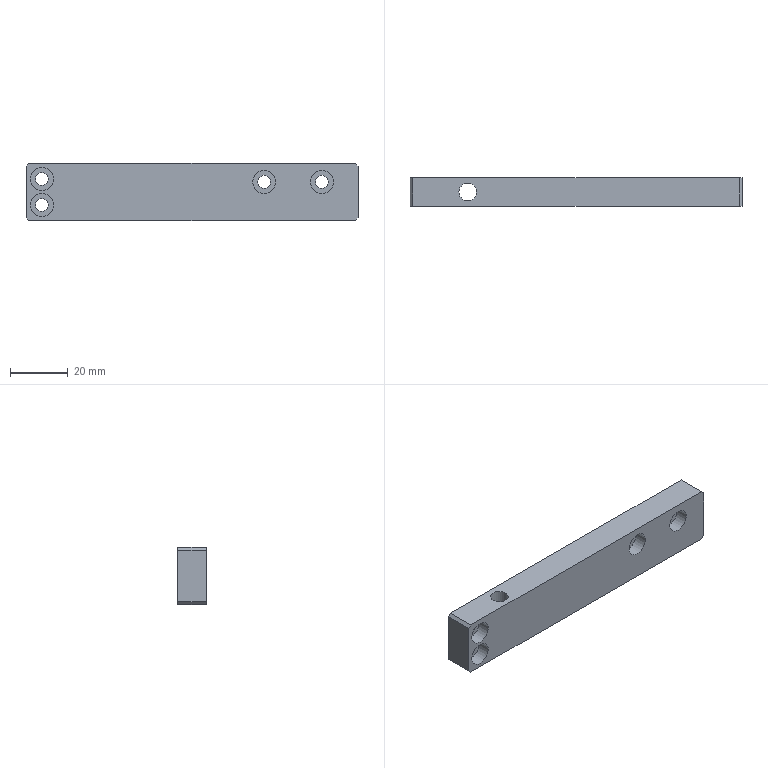Part | NX | 1 solid | 29 faces | box 115 x 10 x 20 mm | volume 20921 mm3 | plane 15 | cylinder 12 | cone 2 | commonest cylinder face diameters 4.5 x4 8 x4 4 x2 6.1 x1 8.2 x1
STEP:
#1=CARTESIAN_POINT('',(-40.55,5.,-8.));
#2=VERTEX_POINT('',#1);
#3=CARTESIAN_POINT('',(-37.5,5.,-8.));
#4=DIRECTION('',(0.,0.,1.));
#5=DIRECTION('',(-1.,0.,0.));
#6=AXIS2_PLACEMENT_3D('',#3,#4,#5);
#7=CIRCLE('',#6,3.05);
#8=EDGE_CURVE('',#2,#2,#7,.T.);
#9=ORIENTED_EDGE('',*,*,#8,.T.);
#10=EDGE_LOOP('',(#9));
#11=FACE_BOUND('',#10,.T.);
#12=CARTESIAN_POINT('',(-41.6,5.,-8.));
#13=VERTEX_POINT('',#12);
#14=CARTESIAN_POINT('',(-37.5,5.,-8.));
#15=DIRECTION('',(0.,0.,-1.));
#16=DIRECTION('',(-1.,0.,0.));
#17=AXIS2_PLACEMENT_3D('',#14,#15,#16);
#18=CIRCLE('',#17,4.1);
#19=EDGE_CURVE('',#13,#13,#18,.T.);
#20=ORIENTED_EDGE('',*,*,#19,.T.);
#21=EDGE_LOOP('',(#20));
#22=FACE_BOUND('',#21,.T.);
#23=CARTESIAN_POINT('',(-37.5,5.,-8.));
#24=DIRECTION('',(0.,0.,-1.));
#25=DIRECTION('',(-1.,0.,0.));
#26=AXIS2_PLACEMENT_3D('',#23,#24,#25);
#27=PLANE('',#26);
#28=ADVANCED_FACE('',(#11,#22),#27,.T.);
#29=CARTESIAN_POINT('',(57.5,10.,-9.));
#30=VERTEX_POINT('',#29);
#31=CARTESIAN_POINT('',(56.5,10.,-10.));
#32=VERTEX_POINT('',#31);
#33=CARTESIAN_POINT('',(56.5,10.,-10.));
#34=DIRECTION('',(-0.7071,0.,-0.7071));
#35=VECTOR('',#34,1000.);
#36=LINE('',#33,#35);
#37=EDGE_CURVE('',#30,#32,#36,.T.);
#38=ORIENTED_EDGE('',*,*,#37,.F.);
#39=CARTESIAN_POINT('',(57.5,0.,-9.));
#40=VERTEX_POINT('',#39);
#41=CARTESIAN_POINT('',(57.5,10.,-9.));
#42=DIRECTION('',(0.,1.,0.));
#43=VECTOR('',#42,1000.);
#44=LINE('',#41,#43);
#45=EDGE_CURVE('',#40,#30,#44,.T.);
#46=ORIENTED_EDGE('',*,*,#45,.F.);
#47=CARTESIAN_POINT('',(56.5,0.,-10.));
#48=VERTEX_POINT('',#47);
#49=CARTESIAN_POINT('',(33.25,0.,-33.25));
#50=DIRECTION('',(0.7071,0.,0.7071));
#51=VECTOR('',#50,1000.);
#52=LINE('',#49,#51);
#53=EDGE_CURVE('',#48,#40,#52,.T.);
#54=ORIENTED_EDGE('',*,*,#53,.F.);
#55=CARTESIAN_POINT('',(56.5,10.,-10.));
#56=DIRECTION('',(0.,-1.,0.));
#57=VECTOR('',#56,1000.);
#58=LINE('',#55,#57);
#59=EDGE_CURVE('',#32,#48,#58,.T.);
#60=ORIENTED_EDGE('',*,*,#59,.F.);
#61=EDGE_LOOP('',(#38,#46,#54,#60));
#62=FACE_BOUND('',#61,.T.);
#63=CARTESIAN_POINT('',(56.5,10.,-10.));
#64=DIRECTION('',(-0.7071,0.,0.7071));
#65=DIRECTION('',(0.,-1.,0.));
#66=AXIS2_PLACEMENT_3D('',#63,#64,#65);
#67=PLANE('',#66);
#68=ADVANCED_FACE('',(#62),#67,.F.);
#69=CARTESIAN_POINT('',(56.5,10.,10.));
#70=VERTEX_POINT('',#69);
#71=CARTESIAN_POINT('',(57.5,10.,9.));
#72=VERTEX_POINT('',#71);
#73=CARTESIAN_POINT('',(57.5,10.,9.));
#74=DIRECTION('',(0.7071,0.,-0.7071));
#75=VECTOR('',#74,1000.);
#76=LINE('',#73,#75);
#77=EDGE_CURVE('',#70,#72,#76,.T.);
#78=ORIENTED_EDGE('',*,*,#77,.F.);
#79=CARTESIAN_POINT('',(56.5,0.,10.));
#80=VERTEX_POINT('',#79);
#81=CARTESIAN_POINT('',(56.5,10.,10.));
#82=DIRECTION('',(0.,1.,0.));
#83=VECTOR('',#82,1000.);
#84=LINE('',#81,#83);
#85=EDGE_CURVE('',#80,#70,#84,.T.);
#86=ORIENTED_EDGE('',*,*,#85,.F.);
#87=CARTESIAN_POINT('',(57.5,0.,9.));
#88=VERTEX_POINT('',#87);
#89=CARTESIAN_POINT('',(33.25,0.,33.25));
#90=DIRECTION('',(-0.7071,0.,0.7071));
#91=VECTOR('',#90,1000.);
#92=LINE('',#89,#91);
#93=EDGE_CURVE('',#88,#80,#92,.T.);
#94=ORIENTED_EDGE('',*,*,#93,.F.);
#95=CARTESIAN_POINT('',(57.5,10.,9.));
#96=DIRECTION('',(0.,-1.,0.));
#97=VECTOR('',#96,1000.);
#98=LINE('',#95,#97);
#99=EDGE_CURVE('',#72,#88,#98,.T.);
#100=ORIENTED_EDGE('',*,*,#99,.F.);
#101=EDGE_LOOP('',(#78,#86,#94,#100));
#102=FACE_BOUND('',#101,.T.);
#103=CARTESIAN_POINT('',(57.5,10.,9.));
#104=DIRECTION('',(-0.7071,0.,-0.7071));
#105=DIRECTION('',(0.,-1.,0.));
#106=AXIS2_PLACEMENT_3D('',#103,#104,#105);
#107=PLANE('',#106);
#108=ADVANCED_FACE('',(#102),#107,.F.);
#109=CARTESIAN_POINT('',(-56.5,10.,-10.));
#110=VERTEX_POINT('',#109);
#111=CARTESIAN_POINT('',(-57.5,10.,-9.));
#112=VERTEX_POINT('',#111);
#113=CARTESIAN_POINT('',(-57.5,10.,-9.));
#114=DIRECTION('',(-0.7071,0.,0.7071));
#115=VECTOR('',#114,1000.);
#116=LINE('',#113,#115);
#117=EDGE_CURVE('',#110,#112,#116,.T.);
#118=ORIENTED_EDGE('',*,*,#117,.F.);
#119=CARTESIAN_POINT('',(-56.5,0.,-10.));
#120=VERTEX_POINT('',#119);
#121=CARTESIAN_POINT('',(-56.5,10.,-10.));
#122=DIRECTION('',(0.,1.,0.));
#123=VECTOR('',#122,1000.);
#124=LINE('',#121,#123);
#125=EDGE_CURVE('',#120,#110,#124,.T.);
#126=ORIENTED_EDGE('',*,*,#125,.F.);
#127=CARTESIAN_POINT('',(-57.5,0.,-9.));
#128=VERTEX_POINT('',#127);
#129=CARTESIAN_POINT('',(-33.25,0.,-33.25));
#130=DIRECTION('',(0.7071,0.,-0.7071));
#131=VECTOR('',#130,1000.);
#132=LINE('',#129,#131);
#133=EDGE_CURVE('',#128,#120,#132,.T.);
#134=ORIENTED_EDGE('',*,*,#133,.F.);
#135=CARTESIAN_POINT('',(-57.5,10.,-9.));
#136=DIRECTION('',(0.,-1.,0.));
#137=VECTOR('',#136,1000.);
#138=LINE('',#135,#137);
#139=EDGE_CURVE('',#112,#128,#138,.T.);
#140=ORIENTED_EDGE('',*,*,#139,.F.);
#141=EDGE_LOOP('',(#118,#126,#134,#140));
#142=FACE_BOUND('',#141,.T.);
#143=CARTESIAN_POINT('',(-57.5,10.,-9.));
#144=DIRECTION('',(0.7071,0.,0.7071));
#145=DIRECTION('',(0.,-1.,0.));
#146=AXIS2_PLACEMENT_3D('',#143,#144,#145);
#147=PLANE('',#146);
#148=ADVANCED_FACE('',(#142),#147,.F.);
#149=CARTESIAN_POINT('',(-57.5,10.,9.));
#150=VERTEX_POINT('',#149);
#151=CARTESIAN_POINT('',(-56.5,10.,10.));
#152=VERTEX_POINT('',#151);
#153=CARTESIAN_POINT('',(-56.5,10.,10.));
#154=DIRECTION('',(0.7071,0.,0.7071));
#155=VECTOR('',#154,1000.);
#156=LINE('',#153,#155);
#157=EDGE_CURVE('',#150,#152,#156,.T.);
#158=ORIENTED_EDGE('',*,*,#157,.F.);
#159=CARTESIAN_POINT('',(-57.5,0.,9.));
#160=VERTEX_POINT('',#159);
#161=CARTESIAN_POINT('',(-57.5,10.,9.));
#162=DIRECTION('',(0.,1.,0.));
#163=VECTOR('',#162,1000.);
#164=LINE('',#161,#163);
#165=EDGE_CURVE('',#160,#150,#164,.T.);
#166=ORIENTED_EDGE('',*,*,#165,.F.);
#167=CARTESIAN_POINT('',(-56.5,0.,10.));
#168=VERTEX_POINT('',#167);
#169=CARTESIAN_POINT('',(-33.25,0.,33.25));
#170=DIRECTION('',(-0.7071,0.,-0.7071));
#171=VECTOR('',#170,1000.);
#172=LINE('',#169,#171);
#173=EDGE_CURVE('',#168,#160,#172,.T.);
#174=ORIENTED_EDGE('',*,*,#173,.F.);
#175=CARTESIAN_POINT('',(-56.5,10.,10.));
#176=DIRECTION('',(0.,-1.,0.));
#177=VECTOR('',#176,1000.);
#178=LINE('',#175,#177);
#179=EDGE_CURVE('',#152,#168,#178,.T.);
#180=ORIENTED_EDGE('',*,*,#179,.F.);
#181=EDGE_LOOP('',(#158,#166,#174,#180));
#182=FACE_BOUND('',#181,.T.);
#183=CARTESIAN_POINT('',(-56.5,10.,10.));
#184=DIRECTION('',(0.7071,0.,-0.7071));
#185=DIRECTION('',(0.,-1.,0.));
#186=AXIS2_PLACEMENT_3D('',#183,#184,#185);
#187=PLANE('',#186);
#188=ADVANCED_FACE('',(#182),#187,.F.);
#189=CARTESIAN_POINT('',(45.,4.4,7.5));
#190=VERTEX_POINT('',#189);
#191=CARTESIAN_POINT('',(45.,4.4,3.5));
#192=DIRECTION('',(0.,-1.,0.));
#193=DIRECTION('',(0.,0.,1.));
#194=AXIS2_PLACEMENT_3D('',#191,#192,#193);
#195=CIRCLE('',#194,4.);
#196=EDGE_CURVE('',#190,#190,#195,.T.);
#197=ORIENTED_EDGE('',*,*,#196,.T.);
#198=EDGE_LOOP('',(#197));
#199=FACE_BOUND('',#198,.T.);
#200=CARTESIAN_POINT('',(45.,4.4,5.75));
#201=VERTEX_POINT('',#200);
#202=CARTESIAN_POINT('',(45.,4.4,3.5));
#203=DIRECTION('',(0.,-1.,0.));
#204=DIRECTION('',(0.,0.,1.));
#205=AXIS2_PLACEMENT_3D('',#202,#203,#204);
#206=CIRCLE('',#205,2.25);
#207=EDGE_CURVE('',#201,#201,#206,.T.);
#208=ORIENTED_EDGE('',*,*,#207,.F.);
#209=EDGE_LOOP('',(#208));
#210=FACE_BOUND('',#209,.T.);
#211=CARTESIAN_POINT('',(-49.75,4.4,4.5));
#212=DIRECTION('',(0.,1.,0.));
#213=DIRECTION('',(0.,0.,1.));
#214=AXIS2_PLACEMENT_3D('',#211,#212,#213);
#215=PLANE('',#214);
#216=ADVANCED_FACE('',(#199,#210),#215,.F.);
#217=CARTESIAN_POINT('',(25.,4.4,7.5));
#218=VERTEX_POINT('',#217);
#219=CARTESIAN_POINT('',(25.,4.4,3.5));
#220=DIRECTION('',(0.,-1.,0.));
#221=DIRECTION('',(0.,0.,1.));
#222=AXIS2_PLACEMENT_3D('',#219,#220,#221);
#223=CIRCLE('',#222,4.);
#224=EDGE_CURVE('',#218,#218,#223,.T.);
#225=ORIENTED_EDGE('',*,*,#224,.T.);
#226=EDGE_LOOP('',(#225));
#227=FACE_BOUND('',#226,.T.);
#228=CARTESIAN_POINT('',(25.,4.4,5.75));
#229=VERTEX_POINT('',#228);
#230=CARTESIAN_POINT('',(25.,4.4,3.5));
#231=DIRECTION('',(0.,-1.,0.));
#232=DIRECTION('',(0.,0.,1.));
#233=AXIS2_PLACEMENT_3D('',#230,#231,#232);
#234=CIRCLE('',#233,2.25);
#235=EDGE_CURVE('',#229,#229,#234,.T.);
#236=ORIENTED_EDGE('',*,*,#235,.F.);
#237=EDGE_LOOP('',(#236));
#238=FACE_BOUND('',#237,.T.);
#239=CARTESIAN_POINT('',(-49.75,4.4,4.5));
#240=DIRECTION('',(0.,1.,0.));
#241=DIRECTION('',(0.,0.,1.));
#242=AXIS2_PLACEMENT_3D('',#239,#240,#241);
#243=PLANE('',#242);
#244=ADVANCED_FACE('',(#227,#238),#243,.F.);
#245=CARTESIAN_POINT('',(-52.,4.4,-0.5));
#246=VERTEX_POINT('',#245);
#247=CARTESIAN_POINT('',(-52.,4.4,-4.5));
#248=DIRECTION('',(0.,-1.,0.));
#249=DIRECTION('',(0.,0.,1.));
#250=AXIS2_PLACEMENT_3D('',#247,#248,#249);
#251=CIRCLE('',#250,4.);
#252=EDGE_CURVE('',#246,#246,#251,.T.);
#253=ORIENTED_EDGE('',*,*,#252,.T.);
#254=EDGE_LOOP('',(#253));
#255=FACE_BOUND('',#254,.T.);
#256=CARTESIAN_POINT('',(-52.,4.4,-2.25));
#257=VERTEX_POINT('',#256);
#258=CARTESIAN_POINT('',(-52.,4.4,-4.5));
#259=DIRECTION('',(0.,-1.,0.));
#260=DIRECTION('',(0.,0.,1.));
#261=AXIS2_PLACEMENT_3D('',#258,#259,#260);
#262=CIRCLE('',#261,2.25);
#263=EDGE_CURVE('',#257,#257,#262,.T.);
#264=ORIENTED_EDGE('',*,*,#263,.F.);
#265=EDGE_LOOP('',(#264));
#266=FACE_BOUND('',#265,.T.);
#267=CARTESIAN_POINT('',(-49.75,4.4,4.5));
#268=DIRECTION('',(0.,1.,0.));
#269=DIRECTION('',(0.,0.,1.));
#270=AXIS2_PLACEMENT_3D('',#267,#268,#269);
#271=PLANE('',#270);
#272=ADVANCED_FACE('',(#255,#266),#271,.F.);
#273=CARTESIAN_POINT('',(-52.,4.4,0.5));
#274=VERTEX_POINT('',#273);
#275=CARTESIAN_POINT('',(-52.,4.4,4.5));
#276=DIRECTION('',(0.,-1.,0.));
#277=DIRECTION('',(0.,0.,-1.));
#278=AXIS2_PLACEMENT_3D('',#275,#276,#277);
#279=CIRCLE('',#278,4.);
#280=EDGE_CURVE('',#274,#274,#279,.T.);
#281=ORIENTED_EDGE('',*,*,#280,.T.);
#282=EDGE_LOOP('',(#281));
#283=FACE_BOUND('',#282,.T.);
#284=CARTESIAN_POINT('',(-52.,4.4,2.25));
#285=VERTEX_POINT('',#284);
#286=CARTESIAN_POINT('',(-52.,4.4,4.5));
#287=DIRECTION('',(0.,-1.,0.));
#288=DIRECTION('',(0.,0.,-1.));
#289=AXIS2_PLACEMENT_3D('',#286,#287,#288);
#290=CIRCLE('',#289,2.25);
#291=EDGE_CURVE('',#285,#285,#290,.T.);
#292=ORIENTED_EDGE('',*,*,#291,.F.);
#293=EDGE_LOOP('',(#292));
#294=FACE_BOUND('',#293,.T.);
#295=CARTESIAN_POINT('',(-49.75,4.4,4.5));
#296=DIRECTION('',(0.,1.,0.));
#297=DIRECTION('',(0.,0.,1.));
#298=AXIS2_PLACEMENT_3D('',#295,#296,#297);
#299=PLANE('',#298);
#300=ADVANCED_FACE('',(#283,#294),#299,.F.);
#301=CARTESIAN_POINT('',(-57.5,0.,10.));
#302=DIRECTION('',(1.,0.,0.));
#303=VECTOR('',#302,1000.);
#304=LINE('',#301,#303);
#305=EDGE_CURVE('',#168,#80,#304,.T.);
#306=ORIENTED_EDGE('',*,*,#305,.F.);
#307=ORIENTED_EDGE('',*,*,#173,.T.);
#308=CARTESIAN_POINT('',(-57.5,0.,10.));
#309=DIRECTION('',(0.,0.,1.));
#310=VECTOR('',#309,1000.);
#311=LINE('',#308,#310);
#312=EDGE_CURVE('',#128,#160,#311,.T.);
#313=ORIENTED_EDGE('',*,*,#312,.F.);
#314=ORIENTED_EDGE('',*,*,#133,.T.);
#315=CARTESIAN_POINT('',(-57.5,0.,-10.));
#316=DIRECTION('',(-1.,0.,0.));
#317=VECTOR('',#316,1000.);
#318=LINE('',#315,#317);
#319=EDGE_CURVE('',#48,#120,#318,.T.);
#320=ORIENTED_EDGE('',*,*,#319,.F.);
#321=ORIENTED_EDGE('',*,*,#53,.T.);
#322=CARTESIAN_POINT('',(57.5,0.,10.));
#323=DIRECTION('',(0.,0.,-1.));
#324=VECTOR('',#323,1000.);
#325=LINE('',#322,#324);
#326=EDGE_CURVE('',#88,#40,#325,.T.);
#327=ORIENTED_EDGE('',*,*,#326,.F.);
#328=ORIENTED_EDGE('',*,*,#93,.T.);
#329=EDGE_LOOP('',(#306,#307,#313,#314,#320,#321,#327,#328));
#330=FACE_BOUND('',#329,.T.);
#331=CARTESIAN_POINT('',(-52.,0.,0.5));
#332=VERTEX_POINT('',#331);
#333=CARTESIAN_POINT('',(-52.,0.,4.5));
#334=DIRECTION('',(0.,-1.,0.));
#335=DIRECTION('',(0.,0.,-1.));
#336=AXIS2_PLACEMENT_3D('',#333,#334,#335);
#337=CIRCLE('',#336,4.);
#338=EDGE_CURVE('',#332,#332,#337,.T.);
#339=ORIENTED_EDGE('',*,*,#338,.F.);
#340=EDGE_LOOP('',(#339));
#341=FACE_BOUND('',#340,.T.);
#342=CARTESIAN_POINT('',(-52.,0.,-8.5));
#343=VERTEX_POINT('',#342);
#344=CARTESIAN_POINT('',(-52.,0.,-4.5));
#345=DIRECTION('',(0.,-1.,0.));
#346=DIRECTION('',(0.,0.,-1.));
#347=AXIS2_PLACEMENT_3D('',#344,#345,#346);
#348=CIRCLE('',#347,4.);
#349=EDGE_CURVE('',#343,#343,#348,.T.);
#350=ORIENTED_EDGE('',*,*,#349,.F.);
#351=EDGE_LOOP('',(#350));
#352=FACE_BOUND('',#351,.T.);
#353=CARTESIAN_POINT('',(25.,0.,-0.5));
#354=VERTEX_POINT('',#353);
#355=CARTESIAN_POINT('',(25.,0.,3.5));
#356=DIRECTION('',(0.,-1.,0.));
#357=DIRECTION('',(0.,0.,-1.));
#358=AXIS2_PLACEMENT_3D('',#355,#356,#357);
#359=CIRCLE('',#358,4.);
#360=EDGE_CURVE('',#354,#354,#359,.T.);
#361=ORIENTED_EDGE('',*,*,#360,.F.);
#362=EDGE_LOOP('',(#361));
#363=FACE_BOUND('',#362,.T.);
#364=CARTESIAN_POINT('',(45.,0.,-0.5));
#365=VERTEX_POINT('',#364);
#366=CARTESIAN_POINT('',(45.,0.,3.5));
#367=DIRECTION('',(0.,-1.,0.));
#368=DIRECTION('',(0.,0.,-1.));
#369=AXIS2_PLACEMENT_3D('',#366,#367,#368);
#370=CIRCLE('',#369,4.);
#371=EDGE_CURVE('',#365,#365,#370,.T.);
#372=ORIENTED_EDGE('',*,*,#371,.F.);
#373=EDGE_LOOP('',(#372));
#374=FACE_BOUND('',#373,.T.);
#375=CARTESIAN_POINT('',(0.,0.,0.));
#376=DIRECTION('',(0.,-1.,0.));
#377=DIRECTION('',(0.,0.,-1.));
#378=AXIS2_PLACEMENT_3D('',#375,#376,#377);
#379=PLANE('',#378);
#380=ADVANCED_FACE('',(#330,#341,#352,#363,#374),#379,.T.);
#381=CARTESIAN_POINT('',(-57.5,10.,10.));
#382=DIRECTION('',(0.,0.,1.));
#383=VECTOR('',#382,1000.);
#384=LINE('',#381,#383);
#385=EDGE_CURVE('',#112,#150,#384,.T.);
#386=ORIENTED_EDGE('',*,*,#385,.T.);
#387=ORIENTED_EDGE('',*,*,#157,.T.);
#388=CARTESIAN_POINT('',(-57.5,10.,10.));
#389=DIRECTION('',(1.,0.,0.));
#390=VECTOR('',#389,1000.);
#391=LINE('',#388,#390);
#392=EDGE_CURVE('',#152,#70,#391,.T.);
#393=ORIENTED_EDGE('',*,*,#392,.T.);
#394=ORIENTED_EDGE('',*,*,#77,.T.);
#395=CARTESIAN_POINT('',(57.5,10.,10.));
#396=DIRECTION('',(0.,0.,-1.));
#397=VECTOR('',#396,1000.);
#398=LINE('',#395,#397);
#399=EDGE_CURVE('',#72,#30,#398,.T.);
#400=ORIENTED_EDGE('',*,*,#399,.T.);
#401=ORIENTED_EDGE('',*,*,#37,.T.);
#402=CARTESIAN_POINT('',(-57.5,10.,-10.));
#403=DIRECTION('',(-1.,0.,0.));
#404=VECTOR('',#403,1000.);
#405=LINE('',#402,#404);
#406=EDGE_CURVE('',#32,#110,#405,.T.);
#407=ORIENTED_EDGE('',*,*,#406,.T.);
#408=ORIENTED_EDGE('',*,*,#117,.T.);
#409=EDGE_LOOP('',(#386,#387,#393,#394,#400,#401,#407,#408));
#410=FACE_BOUND('',#409,.T.);
#411=CARTESIAN_POINT('',(-52.,10.,2.25));
#412=VERTEX_POINT('',#411);
#413=CARTESIAN_POINT('',(-52.,10.,4.5));
#414=DIRECTION('',(0.,-1.,0.));
#415=DIRECTION('',(0.,0.,-1.));
#416=AXIS2_PLACEMENT_3D('',#413,#414,#415);
#417=CIRCLE('',#416,2.25);
#418=EDGE_CURVE('',#412,#412,#417,.T.);
#419=ORIENTED_EDGE('',*,*,#418,.T.);
#420=EDGE_LOOP('',(#419));
#421=FACE_BOUND('',#420,.T.);
#422=CARTESIAN_POINT('',(-52.,10.,-6.75));
#423=VERTEX_POINT('',#422);
#424=CARTESIAN_POINT('',(-52.,10.,-4.5));
#425=DIRECTION('',(0.,-1.,0.));
#426=DIRECTION('',(0.,0.,-1.));
#427=AXIS2_PLACEMENT_3D('',#424,#425,#426);
#428=CIRCLE('',#427,2.25);
#429=EDGE_CURVE('',#423,#423,#428,.T.);
#430=ORIENTED_EDGE('',*,*,#429,.T.);
#431=EDGE_LOOP('',(#430));
#432=FACE_BOUND('',#431,.T.);
#433=CARTESIAN_POINT('',(25.,10.,1.25));
#434=VERTEX_POINT('',#433);
#435=CARTESIAN_POINT('',(25.,10.,3.5));
#436=DIRECTION('',(0.,-1.,0.));
#437=DIRECTION('',(0.,0.,-1.));
#438=AXIS2_PLACEMENT_3D('',#435,#436,#437);
#439=CIRCLE('',#438,2.25);
#440=EDGE_CURVE('',#434,#434,#439,.T.);
#441=ORIENTED_EDGE('',*,*,#440,.T.);
#442=EDGE_LOOP('',(#441));
#443=FACE_BOUND('',#442,.T.);
#444=CARTESIAN_POINT('',(45.,10.,1.25));
#445=VERTEX_POINT('',#444);
#446=CARTESIAN_POINT('',(45.,10.,3.5));
#447=DIRECTION('',(0.,-1.,0.));
#448=DIRECTION('',(0.,0.,-1.));
#449=AXIS2_PLACEMENT_3D('',#446,#447,#448);
#450=CIRCLE('',#449,2.25);
#451=EDGE_CURVE('',#445,#445,#450,.T.);
#452=ORIENTED_EDGE('',*,*,#451,.T.);
#453=EDGE_LOOP('',(#452));
#454=FACE_BOUND('',#453,.T.);
#455=CARTESIAN_POINT('',(25.,10.,-3.5));
#456=VERTEX_POINT('',#455);
#457=CARTESIAN_POINT('',(25.,10.,-5.5));
#458=DIRECTION('',(0.,1.,0.));
#459=DIRECTION('',(0.,0.,1.));
#460=AXIS2_PLACEMENT_3D('',#457,#458,#459);
#461=CIRCLE('',#460,2.);
#462=EDGE_CURVE('',#456,#456,#461,.T.);
#463=ORIENTED_EDGE('',*,*,#462,.F.);
#464=EDGE_LOOP('',(#463));
#465=FACE_BOUND('',#464,.T.);
#466=CARTESIAN_POINT('',(45.,10.,-3.5));
#467=VERTEX_POINT('',#466);
#468=CARTESIAN_POINT('',(45.,10.,-5.5));
#469=DIRECTION('',(0.,1.,0.));
#470=DIRECTION('',(0.,0.,1.));
#471=AXIS2_PLACEMENT_3D('',#468,#469,#470);
#472=CIRCLE('',#471,2.);
#473=EDGE_CURVE('',#467,#467,#472,.T.);
#474=ORIENTED_EDGE('',*,*,#473,.F.);
#475=EDGE_LOOP('',(#474));
#476=FACE_BOUND('',#475,.T.);
#477=CARTESIAN_POINT('',(0.,10.,0.));
#478=DIRECTION('',(0.,-1.,0.));
#479=DIRECTION('',(0.,0.,-1.));
#480=AXIS2_PLACEMENT_3D('',#477,#478,#479);
#481=PLANE('',#480);
#482=ADVANCED_FACE('',(#410,#421,#432,#443,#454,#465,#476),#481,.F.);
#483=ORIENTED_EDGE('',*,*,#392,.F.);
#484=ORIENTED_EDGE('',*,*,#179,.T.);
#485=ORIENTED_EDGE('',*,*,#305,.T.);
#486=ORIENTED_EDGE('',*,*,#85,.T.);
#487=EDGE_LOOP('',(#483,#484,#485,#486));
#488=FACE_BOUND('',#487,.T.);
#489=CARTESIAN_POINT('',(-34.45,5.,10.));
#490=VERTEX_POINT('',#489);
#491=CARTESIAN_POINT('',(-37.5,5.,10.));
#492=DIRECTION('',(0.,0.,1.));
#493=DIRECTION('',(1.,0.,0.));
#494=AXIS2_PLACEMENT_3D('',#491,#492,#493);
#495=CIRCLE('',#494,3.05);
#496=EDGE_CURVE('',#490,#490,#495,.T.);
#497=ORIENTED_EDGE('',*,*,#496,.F.);
#498=EDGE_LOOP('',(#497));
#499=FACE_BOUND('',#498,.T.);
#500=CARTESIAN_POINT('',(-57.5,10.,10.));
#501=DIRECTION('',(0.,0.,-1.));
#502=DIRECTION('',(-1.,0.,0.));
#503=AXIS2_PLACEMENT_3D('',#500,#501,#502);
#504=PLANE('',#503);
#505=ADVANCED_FACE('',(#488,#499),#504,.F.);
#506=ORIENTED_EDGE('',*,*,#312,.T.);
#507=ORIENTED_EDGE('',*,*,#165,.T.);
#508=ORIENTED_EDGE('',*,*,#385,.F.);
#509=ORIENTED_EDGE('',*,*,#139,.T.);
#510=EDGE_LOOP('',(#506,#507,#508,#509));
#511=FACE_BOUND('',#510,.T.);
#512=CARTESIAN_POINT('',(-57.5,10.,10.));
#513=DIRECTION('',(1.,0.,0.));
#514=DIRECTION('',(0.,0.,-1.));
#515=AXIS2_PLACEMENT_3D('',#512,#513,#514);
#516=PLANE('',#515);
#517=ADVANCED_FACE('',(#511),#516,.F.);
#518=ORIENTED_EDGE('',*,*,#319,.T.);
#519=ORIENTED_EDGE('',*,*,#125,.T.);
#520=ORIENTED_EDGE('',*,*,#406,.F.);
#521=ORIENTED_EDGE('',*,*,#59,.T.);
#522=EDGE_LOOP('',(#518,#519,#520,#521));
#523=FACE_BOUND('',#522,.T.);
#524=CARTESIAN_POINT('',(-41.6,5.,-10.));
#525=VERTEX_POINT('',#524);
#526=CARTESIAN_POINT('',(-37.5,5.,-10.));
#527=DIRECTION('',(0.,0.,-1.));
#528=DIRECTION('',(-1.,0.,0.));
#529=AXIS2_PLACEMENT_3D('',#526,#527,#528);
#530=CIRCLE('',#529,4.1);
#531=EDGE_CURVE('',#525,#525,#530,.T.);
#532=ORIENTED_EDGE('',*,*,#531,.F.);
#533=EDGE_LOOP('',(#532));
#534=FACE_BOUND('',#533,.T.);
#535=CARTESIAN_POINT('',(-57.5,10.,-10.));
#536=DIRECTION('',(0.,0.,1.));
#537=DIRECTION('',(1.,0.,0.));
#538=AXIS2_PLACEMENT_3D('',#535,#536,#537);
#539=PLANE('',#538);
#540=ADVANCED_FACE('',(#523,#534),#539,.F.);
#541=ORIENTED_EDGE('',*,*,#399,.F.);
#542=ORIENTED_EDGE('',*,*,#99,.T.);
#543=ORIENTED_EDGE('',*,*,#326,.T.);
#544=ORIENTED_EDGE('',*,*,#45,.T.);
#545=EDGE_LOOP('',(#541,#542,#543,#544));
#546=FACE_BOUND('',#545,.T.);
#547=CARTESIAN_POINT('',(57.5,10.,10.));
#548=DIRECTION('',(-1.,0.,0.));
#549=DIRECTION('',(0.,0.,1.));
#550=AXIS2_PLACEMENT_3D('',#547,#548,#549);
#551=PLANE('',#550);
#552=ADVANCED_FACE('',(#546),#551,.F.);
#553=ORIENTED_EDGE('',*,*,#8,.F.);
#554=EDGE_LOOP('',(#553));
#555=FACE_BOUND('',#554,.T.);
#556=ORIENTED_EDGE('',*,*,#496,.T.);
#557=EDGE_LOOP('',(#556));
#558=FACE_BOUND('',#557,.T.);
#559=CARTESIAN_POINT('',(-37.5,5.,-100.));
#560=DIRECTION('',(0.,0.,1.));
#561=DIRECTION('',(1.,0.,0.));
#562=AXIS2_PLACEMENT_3D('',#559,#560,#561);
#563=CYLINDRICAL_SURFACE('',#562,3.05);
#564=ADVANCED_FACE('',(#555,#558),#563,.F.);
#565=ORIENTED_EDGE('',*,*,#291,.T.);
#566=EDGE_LOOP('',(#565));
#567=FACE_BOUND('',#566,.T.);
#568=ORIENTED_EDGE('',*,*,#418,.F.);
#569=EDGE_LOOP('',(#568));
#570=FACE_BOUND('',#569,.T.);
#571=CARTESIAN_POINT('',(-52.,0.,4.5));
#572=DIRECTION('',(0.,-1.,0.));
#573=DIRECTION('',(0.,0.,-1.));
#574=AXIS2_PLACEMENT_3D('',#571,#572,#573);
#575=CYLINDRICAL_SURFACE('',#574,2.25);
#576=ADVANCED_FACE('',(#567,#570),#575,.F.);
#577=ORIENTED_EDGE('',*,*,#338,.T.);
#578=EDGE_LOOP('',(#577));
#579=FACE_BOUND('',#578,.T.);
#580=ORIENTED_EDGE('',*,*,#280,.F.);
#581=EDGE_LOOP('',(#580));
#582=FACE_BOUND('',#581,.T.);
#583=CARTESIAN_POINT('',(-52.,0.,4.5));
#584=DIRECTION('',(0.,-1.,0.));
#585=DIRECTION('',(0.,0.,-1.));
#586=AXIS2_PLACEMENT_3D('',#583,#584,#585);
#587=CYLINDRICAL_SURFACE('',#586,4.);
#588=ADVANCED_FACE('',(#579,#582),#587,.F.);
#589=ORIENTED_EDGE('',*,*,#263,.T.);
#590=EDGE_LOOP('',(#589));
#591=FACE_BOUND('',#590,.T.);
#592=ORIENTED_EDGE('',*,*,#429,.F.);
#593=EDGE_LOOP('',(#592));
#594=FACE_BOUND('',#593,.T.);
#595=CARTESIAN_POINT('',(-52.,0.,-4.5));
#596=DIRECTION('',(0.,-1.,0.));
#597=DIRECTION('',(0.,0.,-1.));
#598=AXIS2_PLACEMENT_3D('',#595,#596,#597);
#599=CYLINDRICAL_SURFACE('',#598,2.25);
#600=ADVANCED_FACE('',(#591,#594),#599,.F.);
#601=ORIENTED_EDGE('',*,*,#349,.T.);
#602=EDGE_LOOP('',(#601));
#603=FACE_BOUND('',#602,.T.);
#604=ORIENTED_EDGE('',*,*,#252,.F.);
#605=EDGE_LOOP('',(#604));
#606=FACE_BOUND('',#605,.T.);
#607=CARTESIAN_POINT('',(-52.,0.,-4.5));
#608=DIRECTION('',(0.,-1.,0.));
#609=DIRECTION('',(0.,0.,-1.));
#610=AXIS2_PLACEMENT_3D('',#607,#608,#609);
#611=CYLINDRICAL_SURFACE('',#610,4.);
#612=ADVANCED_FACE('',(#603,#606),#611,.F.);
#613=ORIENTED_EDGE('',*,*,#235,.T.);
#614=EDGE_LOOP('',(#613));
#615=FACE_BOUND('',#614,.T.);
#616=ORIENTED_EDGE('',*,*,#440,.F.);
#617=EDGE_LOOP('',(#616));
#618=FACE_BOUND('',#617,.T.);
#619=CARTESIAN_POINT('',(25.,0.,3.5));
#620=DIRECTION('',(0.,-1.,0.));
#621=DIRECTION('',(0.,0.,-1.));
#622=AXIS2_PLACEMENT_3D('',#619,#620,#621);
#623=CYLINDRICAL_SURFACE('',#622,2.25);
#624=ADVANCED_FACE('',(#615,#618),#623,.F.);
#625=ORIENTED_EDGE('',*,*,#360,.T.);
#626=EDGE_LOOP('',(#625));
#627=FACE_BOUND('',#626,.T.);
#628=ORIENTED_EDGE('',*,*,#224,.F.);
#629=EDGE_LOOP('',(#628));
#630=FACE_BOUND('',#629,.T.);
#631=CARTESIAN_POINT('',(25.,0.,3.5));
#632=DIRECTION('',(0.,-1.,0.));
#633=DIRECTION('',(0.,0.,-1.));
#634=AXIS2_PLACEMENT_3D('',#631,#632,#633);
#635=CYLINDRICAL_SURFACE('',#634,4.);
#636=ADVANCED_FACE('',(#627,#630),#635,.F.);
#637=ORIENTED_EDGE('',*,*,#207,.T.);
#638=EDGE_LOOP('',(#637));
#639=FACE_BOUND('',#638,.T.);
#640=ORIENTED_EDGE('',*,*,#451,.F.);
#641=EDGE_LOOP('',(#640));
#642=FACE_BOUND('',#641,.T.);
#643=CARTESIAN_POINT('',(45.,0.,3.5));
#644=DIRECTION('',(0.,-1.,0.));
#645=DIRECTION('',(0.,0.,-1.));
#646=AXIS2_PLACEMENT_3D('',#643,#644,#645);
#647=CYLINDRICAL_SURFACE('',#646,2.25);
#648=ADVANCED_FACE('',(#639,#642),#647,.F.);
#649=ORIENTED_EDGE('',*,*,#371,.T.);
#650=EDGE_LOOP('',(#649));
#651=FACE_BOUND('',#650,.T.);
#652=ORIENTED_EDGE('',*,*,#196,.F.);
#653=EDGE_LOOP('',(#652));
#654=FACE_BOUND('',#653,.T.);
#655=CARTESIAN_POINT('',(45.,0.,3.5));
#656=DIRECTION('',(0.,-1.,0.));
#657=DIRECTION('',(0.,0.,-1.));
#658=AXIS2_PLACEMENT_3D('',#655,#656,#657);
#659=CYLINDRICAL_SURFACE('',#658,4.);
#660=ADVANCED_FACE('',(#651,#654),#659,.F.);
#661=CARTESIAN_POINT('',(25.,3.,-3.5));
#662=VERTEX_POINT('',#661);
#663=CARTESIAN_POINT('',(25.,3.,-5.5));
#664=DIRECTION('',(0.,1.,0.));
#665=DIRECTION('',(0.,0.,1.));
#666=AXIS2_PLACEMENT_3D('',#663,#664,#665);
#667=CIRCLE('',#666,2.);
#668=EDGE_CURVE('',#662,#662,#667,.T.);
#669=ORIENTED_EDGE('',*,*,#668,.T.);
#670=EDGE_LOOP('',(#669));
#671=FACE_BOUND('',#670,.T.);
#672=CARTESIAN_POINT('',(25.,1.798,-5.5));
#673=VERTEX_POINT('',#672);
#674=VERTEX_LOOP('',#673);
#675=FACE_BOUND('',#674,.T.);
#676=CARTESIAN_POINT('',(25.,3.,-5.5));
#677=DIRECTION('',(0.,1.,0.));
#678=DIRECTION('',(0.,0.,1.));
#679=AXIS2_PLACEMENT_3D('',#676,#677,#678);
#680=CONICAL_SURFACE('',#679,2.,1.03);
#681=ADVANCED_FACE('',(#671,#675),#680,.F.);
#682=ORIENTED_EDGE('',*,*,#668,.F.);
#683=EDGE_LOOP('',(#682));
#684=FACE_BOUND('',#683,.T.);
#685=ORIENTED_EDGE('',*,*,#462,.T.);
#686=EDGE_LOOP('',(#685));
#687=FACE_BOUND('',#686,.T.);
#688=CARTESIAN_POINT('',(25.,10.,-5.5));
#689=DIRECTION('',(0.,1.,0.));
#690=DIRECTION('',(0.,0.,1.));
#691=AXIS2_PLACEMENT_3D('',#688,#689,#690);
#692=CYLINDRICAL_SURFACE('',#691,2.);
#693=ADVANCED_FACE('',(#684,#687),#692,.F.);
#694=CARTESIAN_POINT('',(45.,3.,-3.5));
#695=VERTEX_POINT('',#694);
#696=CARTESIAN_POINT('',(45.,3.,-5.5));
#697=DIRECTION('',(0.,1.,0.));
#698=DIRECTION('',(0.,0.,1.));
#699=AXIS2_PLACEMENT_3D('',#696,#697,#698);
#700=CIRCLE('',#699,2.);
#701=EDGE_CURVE('',#695,#695,#700,.T.);
#702=ORIENTED_EDGE('',*,*,#701,.T.);
#703=EDGE_LOOP('',(#702));
#704=FACE_BOUND('',#703,.T.);
#705=CARTESIAN_POINT('',(45.,1.798,-5.5));
#706=VERTEX_POINT('',#705);
#707=VERTEX_LOOP('',#706);
#708=FACE_BOUND('',#707,.T.);
#709=CARTESIAN_POINT('',(45.,3.,-5.5));
#710=DIRECTION('',(0.,1.,0.));
#711=DIRECTION('',(0.,0.,1.));
#712=AXIS2_PLACEMENT_3D('',#709,#710,#711);
#713=CONICAL_SURFACE('',#712,2.,1.03);
#714=ADVANCED_FACE('',(#704,#708),#713,.F.);
#715=ORIENTED_EDGE('',*,*,#701,.F.);
#716=EDGE_LOOP('',(#715));
#717=FACE_BOUND('',#716,.T.);
#718=ORIENTED_EDGE('',*,*,#473,.T.);
#719=EDGE_LOOP('',(#718));
#720=FACE_BOUND('',#719,.T.);
#721=CARTESIAN_POINT('',(45.,10.,-5.5));
#722=DIRECTION('',(0.,1.,0.));
#723=DIRECTION('',(0.,0.,1.));
#724=AXIS2_PLACEMENT_3D('',#721,#722,#723);
#725=CYLINDRICAL_SURFACE('',#724,2.);
#726=ADVANCED_FACE('',(#717,#720),#725,.F.);
#727=ORIENTED_EDGE('',*,*,#531,.T.);
#728=EDGE_LOOP('',(#727));
#729=FACE_BOUND('',#728,.T.);
#730=ORIENTED_EDGE('',*,*,#19,.F.);
#731=EDGE_LOOP('',(#730));
#732=FACE_BOUND('',#731,.T.);
#733=CARTESIAN_POINT('',(-37.5,5.,-8.));
#734=DIRECTION('',(0.,0.,-1.));
#735=DIRECTION('',(-1.,0.,0.));
#736=AXIS2_PLACEMENT_3D('',#733,#734,#735);
#737=CYLINDRICAL_SURFACE('',#736,4.1);
#738=ADVANCED_FACE('',(#729,#732),#737,.F.);
#739=CLOSED_SHELL('',(#28,#68,#108,#148,#188,#216,#244,#272,#300,#380,#482,#505,#517,#540,#552,#564,#576,#588,#600,#612,#624,#636,#648,#660,#681,#693,#714,#726,#738));
#740=MANIFOLD_SOLID_BREP('',#739);
#741=(LENGTH_UNIT()NAMED_UNIT(*)SI_UNIT(.MILLI.,.METRE.));
#742=UNCERTAINTY_MEASURE_WITH_UNIT(LENGTH_MEASURE(0.00001),#741,'','');
#743=(NAMED_UNIT(*)PLANE_ANGLE_UNIT()SI_UNIT($,.RADIAN.));
#744=(NAMED_UNIT(*)SI_UNIT($,.STERADIAN.)SOLID_ANGLE_UNIT());
#745=(GEOMETRIC_REPRESENTATION_CONTEXT(3)GLOBAL_UNCERTAINTY_ASSIGNED_CONTEXT((#742))GLOBAL_UNIT_ASSIGNED_CONTEXT((#741,#743,#744))REPRESENTATION_CONTEXT('',''));
#746=ADVANCED_BREP_SHAPE_REPRESENTATION('',(#740),#745);